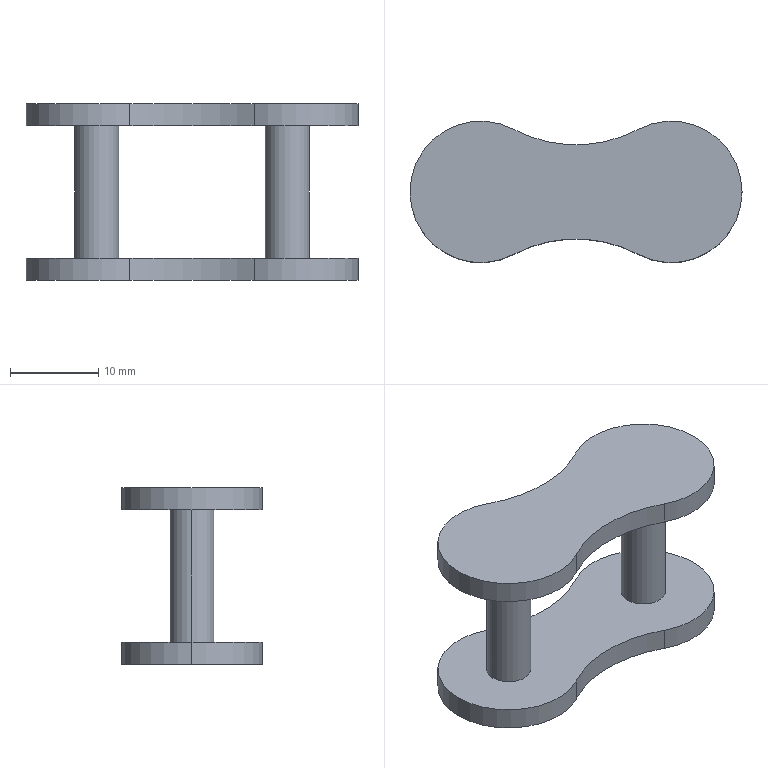Part | SolidWorks | 1 solid | 18 faces | box 37.56 x 16 x 20 mm | volume 2999 mm3 | cylinder 14 | plane 4 | commonest cylinder face diameters 16 x6 5 x4 30 x4
STEP:
#1=CARTESIAN_POINT('',(-8.,0.,-7.5));
#2=VERTEX_POINT('',#1);
#3=CARTESIAN_POINT('',(3.75,-7.067,-7.5));
#4=VERTEX_POINT('',#3);
#5=CARTESIAN_POINT('',(0.,0.,-7.5));
#6=DIRECTION('',(0.,0.,1.));
#7=DIRECTION('',(1.,0.,0.));
#8=AXIS2_PLACEMENT_3D('',#5,#6,#7);
#9=CIRCLE('',#8,8.);
#10=EDGE_CURVE('',#2,#4,#9,.T.);
#11=ORIENTED_EDGE('',*,*,#10,.F.);
#12=CARTESIAN_POINT('',(-8.,0.,-10.));
#13=VERTEX_POINT('',#12);
#14=CARTESIAN_POINT('',(-8.,0.,-7.5));
#15=DIRECTION('',(0.,0.,-1.));
#16=VECTOR('',#15,1000.);
#17=LINE('',#14,#16);
#18=EDGE_CURVE('',#2,#13,#17,.T.);
#19=ORIENTED_EDGE('',*,*,#18,.T.);
#20=CARTESIAN_POINT('',(3.75,-7.067,-10.));
#21=VERTEX_POINT('',#20);
#22=CARTESIAN_POINT('',(0.,0.,-10.));
#23=DIRECTION('',(0.,0.,1.));
#24=DIRECTION('',(1.,0.,0.));
#25=AXIS2_PLACEMENT_3D('',#22,#23,#24);
#26=CIRCLE('',#25,8.);
#27=EDGE_CURVE('',#13,#21,#26,.T.);
#28=ORIENTED_EDGE('',*,*,#27,.T.);
#29=CARTESIAN_POINT('',(3.75,-7.067,-7.5));
#30=DIRECTION('',(0.,0.,-1.));
#31=VECTOR('',#30,1000.);
#32=LINE('',#29,#31);
#33=EDGE_CURVE('',#4,#21,#32,.T.);
#34=ORIENTED_EDGE('',*,*,#33,.F.);
#35=EDGE_LOOP('',(#11,#19,#28,#34));
#36=FACE_OUTER_BOUND('',#35,.T.);
#37=CARTESIAN_POINT('',(0.,0.,-7.5));
#38=DIRECTION('',(0.,0.,-1.));
#39=DIRECTION('',(-1.,0.,0.));
#40=AXIS2_PLACEMENT_3D('',#37,#38,#39);
#41=CYLINDRICAL_SURFACE('',#40,8.);
#42=ADVANCED_FACE('',(#36),#41,.T.);
#43=CARTESIAN_POINT('',(17.81,-7.067,7.5));
#44=VERTEX_POINT('',#43);
#45=CARTESIAN_POINT('',(29.56,0.,7.5));
#46=VERTEX_POINT('',#45);
#47=CARTESIAN_POINT('',(21.56,0.,7.5));
#48=DIRECTION('',(0.,0.,1.));
#49=DIRECTION('',(1.,0.,0.));
#50=AXIS2_PLACEMENT_3D('',#47,#48,#49);
#51=CIRCLE('',#50,8.);
#52=EDGE_CURVE('',#44,#46,#51,.T.);
#53=ORIENTED_EDGE('',*,*,#52,.T.);
#54=CARTESIAN_POINT('',(29.56,0.,10.));
#55=VERTEX_POINT('',#54);
#56=CARTESIAN_POINT('',(29.56,0.,7.5));
#57=DIRECTION('',(0.,0.,1.));
#58=VECTOR('',#57,1000.);
#59=LINE('',#56,#58);
#60=EDGE_CURVE('',#46,#55,#59,.T.);
#61=ORIENTED_EDGE('',*,*,#60,.T.);
#62=CARTESIAN_POINT('',(17.81,-7.067,10.));
#63=VERTEX_POINT('',#62);
#64=CARTESIAN_POINT('',(21.56,0.,10.));
#65=DIRECTION('',(0.,0.,1.));
#66=DIRECTION('',(1.,0.,0.));
#67=AXIS2_PLACEMENT_3D('',#64,#65,#66);
#68=CIRCLE('',#67,8.);
#69=EDGE_CURVE('',#63,#55,#68,.T.);
#70=ORIENTED_EDGE('',*,*,#69,.F.);
#71=CARTESIAN_POINT('',(17.81,-7.067,7.5));
#72=DIRECTION('',(0.,0.,1.));
#73=VECTOR('',#72,1000.);
#74=LINE('',#71,#73);
#75=EDGE_CURVE('',#44,#63,#74,.T.);
#76=ORIENTED_EDGE('',*,*,#75,.F.);
#77=EDGE_LOOP('',(#53,#61,#70,#76));
#78=FACE_OUTER_BOUND('',#77,.T.);
#79=CARTESIAN_POINT('',(21.56,0.,7.5));
#80=DIRECTION('',(0.,0.,1.));
#81=DIRECTION('',(1.,0.,0.));
#82=AXIS2_PLACEMENT_3D('',#79,#80,#81);
#83=CYLINDRICAL_SURFACE('',#82,8.);
#84=ADVANCED_FACE('',(#78),#83,.T.);
#85=CARTESIAN_POINT('',(19.06,0.,7.5));
#86=VERTEX_POINT('',#85);
#87=CARTESIAN_POINT('',(24.06,0.,7.5));
#88=VERTEX_POINT('',#87);
#89=CARTESIAN_POINT('',(21.56,0.,7.5));
#90=DIRECTION('',(0.,0.,-1.));
#91=DIRECTION('',(1.,0.,0.));
#92=AXIS2_PLACEMENT_3D('',#89,#90,#91);
#93=CIRCLE('',#92,2.5);
#94=EDGE_CURVE('',#86,#88,#93,.T.);
#95=ORIENTED_EDGE('',*,*,#94,.T.);
#96=CARTESIAN_POINT('',(24.06,0.,-7.5));
#97=VERTEX_POINT('',#96);
#98=CARTESIAN_POINT('',(24.06,0.,10.));
#99=DIRECTION('',(0.,0.,-1.));
#100=VECTOR('',#99,1000.);
#101=LINE('',#98,#100);
#102=EDGE_CURVE('',#88,#97,#101,.T.);
#103=ORIENTED_EDGE('',*,*,#102,.T.);
#104=CARTESIAN_POINT('',(19.06,0.,-7.5));
#105=VERTEX_POINT('',#104);
#106=CARTESIAN_POINT('',(21.56,0.,-7.5));
#107=DIRECTION('',(0.,0.,-1.));
#108=DIRECTION('',(-1.,0.,0.));
#109=AXIS2_PLACEMENT_3D('',#106,#107,#108);
#110=CIRCLE('',#109,2.5);
#111=EDGE_CURVE('',#105,#97,#110,.T.);
#112=ORIENTED_EDGE('',*,*,#111,.F.);
#113=CARTESIAN_POINT('',(19.06,0.,10.));
#114=DIRECTION('',(0.,0.,-1.));
#115=VECTOR('',#114,1000.);
#116=LINE('',#113,#115);
#117=EDGE_CURVE('',#86,#105,#116,.T.);
#118=ORIENTED_EDGE('',*,*,#117,.F.);
#119=EDGE_LOOP('',(#95,#103,#112,#118));
#120=FACE_OUTER_BOUND('',#119,.T.);
#121=CARTESIAN_POINT('',(21.56,0.,10.));
#122=DIRECTION('',(0.,0.,-1.));
#123=DIRECTION('',(-1.,0.,0.));
#124=AXIS2_PLACEMENT_3D('',#121,#122,#123);
#125=CYLINDRICAL_SURFACE('',#124,2.5);
#126=ADVANCED_FACE('',(#120),#125,.T.);
#127=CARTESIAN_POINT('',(2.5,0.,7.5));
#128=VERTEX_POINT('',#127);
#129=CARTESIAN_POINT('',(-2.5,0.,7.5));
#130=VERTEX_POINT('',#129);
#131=CARTESIAN_POINT('',(0.,0.,7.5));
#132=DIRECTION('',(0.,0.,1.));
#133=DIRECTION('',(1.,0.,0.));
#134=AXIS2_PLACEMENT_3D('',#131,#132,#133);
#135=CIRCLE('',#134,2.5);
#136=EDGE_CURVE('',#128,#130,#135,.T.);
#137=ORIENTED_EDGE('',*,*,#136,.F.);
#138=CARTESIAN_POINT('',(2.5,0.,-7.5));
#139=VERTEX_POINT('',#138);
#140=CARTESIAN_POINT('',(2.5,0.,10.));
#141=DIRECTION('',(0.,0.,-1.));
#142=VECTOR('',#141,1000.);
#143=LINE('',#140,#142);
#144=EDGE_CURVE('',#128,#139,#143,.T.);
#145=ORIENTED_EDGE('',*,*,#144,.T.);
#146=CARTESIAN_POINT('',(-2.5,0.,-7.5));
#147=VERTEX_POINT('',#146);
#148=CARTESIAN_POINT('',(0.,0.,-7.5));
#149=DIRECTION('',(0.,0.,-1.));
#150=DIRECTION('',(-1.,0.,0.));
#151=AXIS2_PLACEMENT_3D('',#148,#149,#150);
#152=CIRCLE('',#151,2.5);
#153=EDGE_CURVE('',#147,#139,#152,.T.);
#154=ORIENTED_EDGE('',*,*,#153,.F.);
#155=CARTESIAN_POINT('',(-2.5,0.,10.));
#156=DIRECTION('',(0.,0.,-1.));
#157=VECTOR('',#156,1000.);
#158=LINE('',#155,#157);
#159=EDGE_CURVE('',#130,#147,#158,.T.);
#160=ORIENTED_EDGE('',*,*,#159,.F.);
#161=EDGE_LOOP('',(#137,#145,#154,#160));
#162=FACE_OUTER_BOUND('',#161,.T.);
#163=CARTESIAN_POINT('',(0.,0.,10.));
#164=DIRECTION('',(0.,0.,-1.));
#165=DIRECTION('',(-1.,0.,0.));
#166=AXIS2_PLACEMENT_3D('',#163,#164,#165);
#167=CYLINDRICAL_SURFACE('',#166,2.5);
#168=ADVANCED_FACE('',(#162),#167,.T.);
#169=ORIENTED_EDGE('',*,*,#144,.F.);
#170=CARTESIAN_POINT('',(0.,0.,7.5));
#171=DIRECTION('',(0.,0.,1.));
#172=DIRECTION('',(1.,0.,0.));
#173=AXIS2_PLACEMENT_3D('',#170,#171,#172);
#174=CIRCLE('',#173,2.5);
#175=EDGE_CURVE('',#130,#128,#174,.T.);
#176=ORIENTED_EDGE('',*,*,#175,.F.);
#177=ORIENTED_EDGE('',*,*,#159,.T.);
#178=CARTESIAN_POINT('',(0.,0.,-7.5));
#179=DIRECTION('',(0.,0.,-1.));
#180=DIRECTION('',(-1.,0.,0.));
#181=AXIS2_PLACEMENT_3D('',#178,#179,#180);
#182=CIRCLE('',#181,2.5);
#183=EDGE_CURVE('',#139,#147,#182,.T.);
#184=ORIENTED_EDGE('',*,*,#183,.F.);
#185=EDGE_LOOP('',(#169,#176,#177,#184));
#186=FACE_OUTER_BOUND('',#185,.T.);
#187=CARTESIAN_POINT('',(0.,0.,10.));
#188=DIRECTION('',(0.,0.,-1.));
#189=DIRECTION('',(-1.,0.,0.));
#190=AXIS2_PLACEMENT_3D('',#187,#188,#189);
#191=CYLINDRICAL_SURFACE('',#190,2.5);
#192=ADVANCED_FACE('',(#186),#191,.T.);
#193=ORIENTED_EDGE('',*,*,#102,.F.);
#194=CARTESIAN_POINT('',(21.56,0.,7.5));
#195=DIRECTION('',(0.,0.,-1.));
#196=DIRECTION('',(1.,0.,0.));
#197=AXIS2_PLACEMENT_3D('',#194,#195,#196);
#198=CIRCLE('',#197,2.5);
#199=EDGE_CURVE('',#88,#86,#198,.T.);
#200=ORIENTED_EDGE('',*,*,#199,.T.);
#201=ORIENTED_EDGE('',*,*,#117,.T.);
#202=CARTESIAN_POINT('',(21.56,0.,-7.5));
#203=DIRECTION('',(0.,0.,-1.));
#204=DIRECTION('',(-1.,0.,0.));
#205=AXIS2_PLACEMENT_3D('',#202,#203,#204);
#206=CIRCLE('',#205,2.5);
#207=EDGE_CURVE('',#97,#105,#206,.T.);
#208=ORIENTED_EDGE('',*,*,#207,.F.);
#209=EDGE_LOOP('',(#193,#200,#201,#208));
#210=FACE_OUTER_BOUND('',#209,.T.);
#211=CARTESIAN_POINT('',(21.56,0.,10.));
#212=DIRECTION('',(0.,0.,-1.));
#213=DIRECTION('',(-1.,0.,0.));
#214=AXIS2_PLACEMENT_3D('',#211,#212,#213);
#215=CYLINDRICAL_SURFACE('',#214,2.5);
#216=ADVANCED_FACE('',(#210),#215,.T.);
#217=ORIENTED_EDGE('',*,*,#60,.F.);
#218=CARTESIAN_POINT('',(17.81,7.067,7.5));
#219=VERTEX_POINT('',#218);
#220=CARTESIAN_POINT('',(21.56,0.,7.5));
#221=DIRECTION('',(0.,0.,1.));
#222=DIRECTION('',(1.,0.,0.));
#223=AXIS2_PLACEMENT_3D('',#220,#221,#222);
#224=CIRCLE('',#223,8.);
#225=EDGE_CURVE('',#46,#219,#224,.T.);
#226=ORIENTED_EDGE('',*,*,#225,.T.);
#227=CARTESIAN_POINT('',(17.81,7.067,10.));
#228=VERTEX_POINT('',#227);
#229=CARTESIAN_POINT('',(17.81,7.067,7.5));
#230=DIRECTION('',(0.,0.,1.));
#231=VECTOR('',#230,1000.);
#232=LINE('',#229,#231);
#233=EDGE_CURVE('',#219,#228,#232,.T.);
#234=ORIENTED_EDGE('',*,*,#233,.T.);
#235=CARTESIAN_POINT('',(21.56,0.,10.));
#236=DIRECTION('',(0.,0.,1.));
#237=DIRECTION('',(1.,0.,0.));
#238=AXIS2_PLACEMENT_3D('',#235,#236,#237);
#239=CIRCLE('',#238,8.);
#240=EDGE_CURVE('',#55,#228,#239,.T.);
#241=ORIENTED_EDGE('',*,*,#240,.F.);
#242=EDGE_LOOP('',(#217,#226,#234,#241));
#243=FACE_OUTER_BOUND('',#242,.T.);
#244=CARTESIAN_POINT('',(21.56,0.,7.5));
#245=DIRECTION('',(0.,0.,1.));
#246=DIRECTION('',(1.,0.,0.));
#247=AXIS2_PLACEMENT_3D('',#244,#245,#246);
#248=CYLINDRICAL_SURFACE('',#247,8.);
#249=ADVANCED_FACE('',(#243),#248,.T.);
#250=CARTESIAN_POINT('',(3.75,-7.067,10.));
#251=VERTEX_POINT('',#250);
#252=CARTESIAN_POINT('',(10.78,-20.317,10.));
#253=DIRECTION('',(0.,0.,-1.));
#254=DIRECTION('',(1.,0.,0.));
#255=AXIS2_PLACEMENT_3D('',#252,#253,#254);
#256=CIRCLE('',#255,15.);
#257=EDGE_CURVE('',#251,#63,#256,.T.);
#258=ORIENTED_EDGE('',*,*,#257,.F.);
#259=CARTESIAN_POINT('',(3.75,-7.067,7.5));
#260=VERTEX_POINT('',#259);
#261=CARTESIAN_POINT('',(3.75,-7.067,7.5));
#262=DIRECTION('',(0.,0.,1.));
#263=VECTOR('',#262,1000.);
#264=LINE('',#261,#263);
#265=EDGE_CURVE('',#260,#251,#264,.T.);
#266=ORIENTED_EDGE('',*,*,#265,.F.);
#267=CARTESIAN_POINT('',(10.78,-20.317,7.5));
#268=DIRECTION('',(0.,0.,-1.));
#269=DIRECTION('',(1.,0.,0.));
#270=AXIS2_PLACEMENT_3D('',#267,#268,#269);
#271=CIRCLE('',#270,15.);
#272=EDGE_CURVE('',#260,#44,#271,.T.);
#273=ORIENTED_EDGE('',*,*,#272,.T.);
#274=ORIENTED_EDGE('',*,*,#75,.T.);
#275=EDGE_LOOP('',(#258,#266,#273,#274));
#276=FACE_OUTER_BOUND('',#275,.T.);
#277=CARTESIAN_POINT('',(10.78,-20.317,7.5));
#278=DIRECTION('',(0.,0.,1.));
#279=DIRECTION('',(1.,0.,0.));
#280=AXIS2_PLACEMENT_3D('',#277,#278,#279);
#281=CYLINDRICAL_SURFACE('',#280,15.);
#282=ADVANCED_FACE('',(#276),#281,.F.);
#283=CARTESIAN_POINT('',(3.75,7.067,10.));
#284=VERTEX_POINT('',#283);
#285=CARTESIAN_POINT('',(0.,0.,10.));
#286=DIRECTION('',(0.,0.,1.));
#287=DIRECTION('',(1.,0.,0.));
#288=AXIS2_PLACEMENT_3D('',#285,#286,#287);
#289=CIRCLE('',#288,8.);
#290=EDGE_CURVE('',#284,#251,#289,.T.);
#291=ORIENTED_EDGE('',*,*,#290,.F.);
#292=CARTESIAN_POINT('',(3.75,7.067,7.5));
#293=VERTEX_POINT('',#292);
#294=CARTESIAN_POINT('',(3.75,7.067,7.5));
#295=DIRECTION('',(0.,0.,1.));
#296=VECTOR('',#295,1000.);
#297=LINE('',#294,#296);
#298=EDGE_CURVE('',#293,#284,#297,.T.);
#299=ORIENTED_EDGE('',*,*,#298,.F.);
#300=CARTESIAN_POINT('',(0.,0.,7.5));
#301=DIRECTION('',(0.,0.,1.));
#302=DIRECTION('',(1.,0.,0.));
#303=AXIS2_PLACEMENT_3D('',#300,#301,#302);
#304=CIRCLE('',#303,8.);
#305=EDGE_CURVE('',#293,#260,#304,.T.);
#306=ORIENTED_EDGE('',*,*,#305,.T.);
#307=ORIENTED_EDGE('',*,*,#265,.T.);
#308=EDGE_LOOP('',(#291,#299,#306,#307));
#309=FACE_OUTER_BOUND('',#308,.T.);
#310=CARTESIAN_POINT('',(0.,0.,7.5));
#311=DIRECTION('',(0.,0.,1.));
#312=DIRECTION('',(1.,0.,0.));
#313=AXIS2_PLACEMENT_3D('',#310,#311,#312);
#314=CYLINDRICAL_SURFACE('',#313,8.);
#315=ADVANCED_FACE('',(#309),#314,.T.);
#316=CARTESIAN_POINT('',(10.78,20.317,10.));
#317=DIRECTION('',(0.,0.,1.));
#318=DIRECTION('',(1.,0.,0.));
#319=AXIS2_PLACEMENT_3D('',#316,#317,#318);
#320=CIRCLE('',#319,15.);
#321=EDGE_CURVE('',#284,#228,#320,.T.);
#322=ORIENTED_EDGE('',*,*,#321,.T.);
#323=ORIENTED_EDGE('',*,*,#233,.F.);
#324=CARTESIAN_POINT('',(10.78,20.317,7.5));
#325=DIRECTION('',(0.,0.,1.));
#326=DIRECTION('',(1.,0.,0.));
#327=AXIS2_PLACEMENT_3D('',#324,#325,#326);
#328=CIRCLE('',#327,15.);
#329=EDGE_CURVE('',#293,#219,#328,.T.);
#330=ORIENTED_EDGE('',*,*,#329,.F.);
#331=ORIENTED_EDGE('',*,*,#298,.T.);
#332=EDGE_LOOP('',(#322,#323,#330,#331));
#333=FACE_OUTER_BOUND('',#332,.T.);
#334=CARTESIAN_POINT('',(10.78,20.317,7.5));
#335=DIRECTION('',(0.,0.,1.));
#336=DIRECTION('',(1.,0.,0.));
#337=AXIS2_PLACEMENT_3D('',#334,#335,#336);
#338=CYLINDRICAL_SURFACE('',#337,15.);
#339=ADVANCED_FACE('',(#333),#338,.F.);
#340=ORIENTED_EDGE('',*,*,#94,.F.);
#341=ORIENTED_EDGE('',*,*,#199,.F.);
#342=EDGE_LOOP('',(#340,#341));
#343=FACE_BOUND('',#342,.T.);
#344=ORIENTED_EDGE('',*,*,#52,.F.);
#345=ORIENTED_EDGE('',*,*,#272,.F.);
#346=ORIENTED_EDGE('',*,*,#305,.F.);
#347=ORIENTED_EDGE('',*,*,#329,.T.);
#348=ORIENTED_EDGE('',*,*,#225,.F.);
#349=EDGE_LOOP('',(#344,#345,#346,#347,#348));
#350=FACE_OUTER_BOUND('',#349,.T.);
#351=ORIENTED_EDGE('',*,*,#175,.T.);
#352=ORIENTED_EDGE('',*,*,#136,.T.);
#353=EDGE_LOOP('',(#351,#352));
#354=FACE_BOUND('',#353,.T.);
#355=CARTESIAN_POINT('',(0.,0.,7.5));
#356=DIRECTION('',(0.,0.,1.));
#357=DIRECTION('',(1.,0.,0.));
#358=AXIS2_PLACEMENT_3D('',#355,#356,#357);
#359=PLANE('',#358);
#360=ADVANCED_FACE('',(#343,#350,#354),#359,.F.);
#361=ORIENTED_EDGE('',*,*,#69,.T.);
#362=ORIENTED_EDGE('',*,*,#240,.T.);
#363=ORIENTED_EDGE('',*,*,#321,.F.);
#364=ORIENTED_EDGE('',*,*,#290,.T.);
#365=ORIENTED_EDGE('',*,*,#257,.T.);
#366=EDGE_LOOP('',(#361,#362,#363,#364,#365));
#367=FACE_OUTER_BOUND('',#366,.T.);
#368=CARTESIAN_POINT('',(0.,0.,10.));
#369=DIRECTION('',(0.,0.,1.));
#370=DIRECTION('',(1.,0.,0.));
#371=AXIS2_PLACEMENT_3D('',#368,#369,#370);
#372=PLANE('',#371);
#373=ADVANCED_FACE('',(#367),#372,.T.);
#374=CARTESIAN_POINT('',(17.81,-7.067,-10.));
#375=VERTEX_POINT('',#374);
#376=CARTESIAN_POINT('',(17.81,7.067,-10.));
#377=VERTEX_POINT('',#376);
#378=CARTESIAN_POINT('',(21.56,0.,-10.));
#379=DIRECTION('',(0.,0.,1.));
#380=DIRECTION('',(1.,0.,0.));
#381=AXIS2_PLACEMENT_3D('',#378,#379,#380);
#382=CIRCLE('',#381,8.);
#383=EDGE_CURVE('',#375,#377,#382,.T.);
#384=ORIENTED_EDGE('',*,*,#383,.T.);
#385=CARTESIAN_POINT('',(17.81,7.067,-7.5));
#386=VERTEX_POINT('',#385);
#387=CARTESIAN_POINT('',(17.81,7.067,-7.5));
#388=DIRECTION('',(0.,0.,-1.));
#389=VECTOR('',#388,1000.);
#390=LINE('',#387,#389);
#391=EDGE_CURVE('',#386,#377,#390,.T.);
#392=ORIENTED_EDGE('',*,*,#391,.F.);
#393=CARTESIAN_POINT('',(17.81,-7.067,-7.5));
#394=VERTEX_POINT('',#393);
#395=CARTESIAN_POINT('',(21.56,0.,-7.5));
#396=DIRECTION('',(0.,0.,1.));
#397=DIRECTION('',(1.,0.,0.));
#398=AXIS2_PLACEMENT_3D('',#395,#396,#397);
#399=CIRCLE('',#398,8.);
#400=EDGE_CURVE('',#394,#386,#399,.T.);
#401=ORIENTED_EDGE('',*,*,#400,.F.);
#402=CARTESIAN_POINT('',(17.81,-7.067,-7.5));
#403=DIRECTION('',(0.,0.,-1.));
#404=VECTOR('',#403,1000.);
#405=LINE('',#402,#404);
#406=EDGE_CURVE('',#394,#375,#405,.T.);
#407=ORIENTED_EDGE('',*,*,#406,.T.);
#408=EDGE_LOOP('',(#384,#392,#401,#407));
#409=FACE_OUTER_BOUND('',#408,.T.);
#410=CARTESIAN_POINT('',(21.56,0.,-7.5));
#411=DIRECTION('',(0.,0.,-1.));
#412=DIRECTION('',(-1.,0.,0.));
#413=AXIS2_PLACEMENT_3D('',#410,#411,#412);
#414=CYLINDRICAL_SURFACE('',#413,8.);
#415=ADVANCED_FACE('',(#409),#414,.T.);
#416=CARTESIAN_POINT('',(3.75,7.067,-10.));
#417=VERTEX_POINT('',#416);
#418=CARTESIAN_POINT('',(10.78,20.317,-10.));
#419=DIRECTION('',(0.,0.,1.));
#420=DIRECTION('',(1.,0.,0.));
#421=AXIS2_PLACEMENT_3D('',#418,#419,#420);
#422=CIRCLE('',#421,15.);
#423=EDGE_CURVE('',#417,#377,#422,.T.);
#424=ORIENTED_EDGE('',*,*,#423,.F.);
#425=CARTESIAN_POINT('',(3.75,7.067,-7.5));
#426=VERTEX_POINT('',#425);
#427=CARTESIAN_POINT('',(3.75,7.067,-7.5));
#428=DIRECTION('',(0.,0.,-1.));
#429=VECTOR('',#428,1000.);
#430=LINE('',#427,#429);
#431=EDGE_CURVE('',#426,#417,#430,.T.);
#432=ORIENTED_EDGE('',*,*,#431,.F.);
#433=CARTESIAN_POINT('',(10.78,20.317,-7.5));
#434=DIRECTION('',(0.,0.,1.));
#435=DIRECTION('',(1.,0.,0.));
#436=AXIS2_PLACEMENT_3D('',#433,#434,#435);
#437=CIRCLE('',#436,15.);
#438=EDGE_CURVE('',#426,#386,#437,.T.);
#439=ORIENTED_EDGE('',*,*,#438,.T.);
#440=ORIENTED_EDGE('',*,*,#391,.T.);
#441=EDGE_LOOP('',(#424,#432,#439,#440));
#442=FACE_OUTER_BOUND('',#441,.T.);
#443=CARTESIAN_POINT('',(10.78,20.317,-7.5));
#444=DIRECTION('',(0.,0.,-1.));
#445=DIRECTION('',(-1.,0.,0.));
#446=AXIS2_PLACEMENT_3D('',#443,#444,#445);
#447=CYLINDRICAL_SURFACE('',#446,15.);
#448=ADVANCED_FACE('',(#442),#447,.F.);
#449=ORIENTED_EDGE('',*,*,#18,.F.);
#450=CARTESIAN_POINT('',(0.,0.,-7.5));
#451=DIRECTION('',(0.,0.,1.));
#452=DIRECTION('',(1.,0.,0.));
#453=AXIS2_PLACEMENT_3D('',#450,#451,#452);
#454=CIRCLE('',#453,8.);
#455=EDGE_CURVE('',#426,#2,#454,.T.);
#456=ORIENTED_EDGE('',*,*,#455,.F.);
#457=ORIENTED_EDGE('',*,*,#431,.T.);
#458=CARTESIAN_POINT('',(0.,0.,-10.));
#459=DIRECTION('',(0.,0.,1.));
#460=DIRECTION('',(1.,0.,0.));
#461=AXIS2_PLACEMENT_3D('',#458,#459,#460);
#462=CIRCLE('',#461,8.);
#463=EDGE_CURVE('',#417,#13,#462,.T.);
#464=ORIENTED_EDGE('',*,*,#463,.T.);
#465=EDGE_LOOP('',(#449,#456,#457,#464));
#466=FACE_OUTER_BOUND('',#465,.T.);
#467=CARTESIAN_POINT('',(0.,0.,-7.5));
#468=DIRECTION('',(0.,0.,-1.));
#469=DIRECTION('',(-1.,0.,0.));
#470=AXIS2_PLACEMENT_3D('',#467,#468,#469);
#471=CYLINDRICAL_SURFACE('',#470,8.);
#472=ADVANCED_FACE('',(#466),#471,.T.);
#473=CARTESIAN_POINT('',(10.78,-20.317,-10.));
#474=DIRECTION('',(0.,0.,-1.));
#475=DIRECTION('',(1.,0.,0.));
#476=AXIS2_PLACEMENT_3D('',#473,#474,#475);
#477=CIRCLE('',#476,15.);
#478=EDGE_CURVE('',#21,#375,#477,.T.);
#479=ORIENTED_EDGE('',*,*,#478,.T.);
#480=ORIENTED_EDGE('',*,*,#406,.F.);
#481=CARTESIAN_POINT('',(10.78,-20.317,-7.5));
#482=DIRECTION('',(0.,0.,-1.));
#483=DIRECTION('',(1.,0.,0.));
#484=AXIS2_PLACEMENT_3D('',#481,#482,#483);
#485=CIRCLE('',#484,15.);
#486=EDGE_CURVE('',#4,#394,#485,.T.);
#487=ORIENTED_EDGE('',*,*,#486,.F.);
#488=ORIENTED_EDGE('',*,*,#33,.T.);
#489=EDGE_LOOP('',(#479,#480,#487,#488));
#490=FACE_OUTER_BOUND('',#489,.T.);
#491=CARTESIAN_POINT('',(10.78,-20.317,-7.5));
#492=DIRECTION('',(0.,0.,-1.));
#493=DIRECTION('',(-1.,0.,0.));
#494=AXIS2_PLACEMENT_3D('',#491,#492,#493);
#495=CYLINDRICAL_SURFACE('',#494,15.);
#496=ADVANCED_FACE('',(#490),#495,.F.);
#497=ORIENTED_EDGE('',*,*,#111,.T.);
#498=ORIENTED_EDGE('',*,*,#207,.T.);
#499=EDGE_LOOP('',(#497,#498));
#500=FACE_BOUND('',#499,.T.);
#501=ORIENTED_EDGE('',*,*,#400,.T.);
#502=ORIENTED_EDGE('',*,*,#438,.F.);
#503=ORIENTED_EDGE('',*,*,#455,.T.);
#504=ORIENTED_EDGE('',*,*,#10,.T.);
#505=ORIENTED_EDGE('',*,*,#486,.T.);
#506=EDGE_LOOP('',(#501,#502,#503,#504,#505));
#507=FACE_OUTER_BOUND('',#506,.T.);
#508=ORIENTED_EDGE('',*,*,#153,.T.);
#509=ORIENTED_EDGE('',*,*,#183,.T.);
#510=EDGE_LOOP('',(#508,#509));
#511=FACE_BOUND('',#510,.T.);
#512=CARTESIAN_POINT('',(0.,0.,-7.5));
#513=DIRECTION('',(0.,0.,-1.));
#514=DIRECTION('',(1.,0.,0.));
#515=AXIS2_PLACEMENT_3D('',#512,#513,#514);
#516=PLANE('',#515);
#517=ADVANCED_FACE('',(#500,#507,#511),#516,.F.);
#518=ORIENTED_EDGE('',*,*,#383,.F.);
#519=ORIENTED_EDGE('',*,*,#478,.F.);
#520=ORIENTED_EDGE('',*,*,#27,.F.);
#521=ORIENTED_EDGE('',*,*,#463,.F.);
#522=ORIENTED_EDGE('',*,*,#423,.T.);
#523=EDGE_LOOP('',(#518,#519,#520,#521,#522));
#524=FACE_OUTER_BOUND('',#523,.T.);
#525=CARTESIAN_POINT('',(0.,0.,-10.));
#526=DIRECTION('',(0.,0.,1.));
#527=DIRECTION('',(1.,0.,0.));
#528=AXIS2_PLACEMENT_3D('',#525,#526,#527);
#529=PLANE('',#528);
#530=ADVANCED_FACE('',(#524),#529,.F.);
#531=CLOSED_SHELL('',(#42,#84,#126,#168,#192,#216,#249,#282,#315,#339,#360,#373,#415,#448,#472,#496,#517,#530));
#532=MANIFOLD_SOLID_BREP('',#531);
#533=CARTESIAN_POINT('',(0.,0.,0.));
#534=DIRECTION('',(0.,0.,1.));
#535=DIRECTION('',(1.,0.,0.));
#536=AXIS2_PLACEMENT_3D('',#533,#534,#535);
#537=(LENGTH_UNIT()NAMED_UNIT(*)SI_UNIT(.MILLI.,.METRE.));
#538=UNCERTAINTY_MEASURE_WITH_UNIT(LENGTH_MEASURE(0.00001),#537,'','');
#539=(NAMED_UNIT(*)PLANE_ANGLE_UNIT()SI_UNIT($,.RADIAN.));
#540=(NAMED_UNIT(*)SI_UNIT($,.STERADIAN.)SOLID_ANGLE_UNIT());
#541=(GEOMETRIC_REPRESENTATION_CONTEXT(3)GLOBAL_UNCERTAINTY_ASSIGNED_CONTEXT((#538))GLOBAL_UNIT_ASSIGNED_CONTEXT((#537,#539,#540))REPRESENTATION_CONTEXT('',''));
#542=ADVANCED_BREP_SHAPE_REPRESENTATION('',(#532,#536),#541);